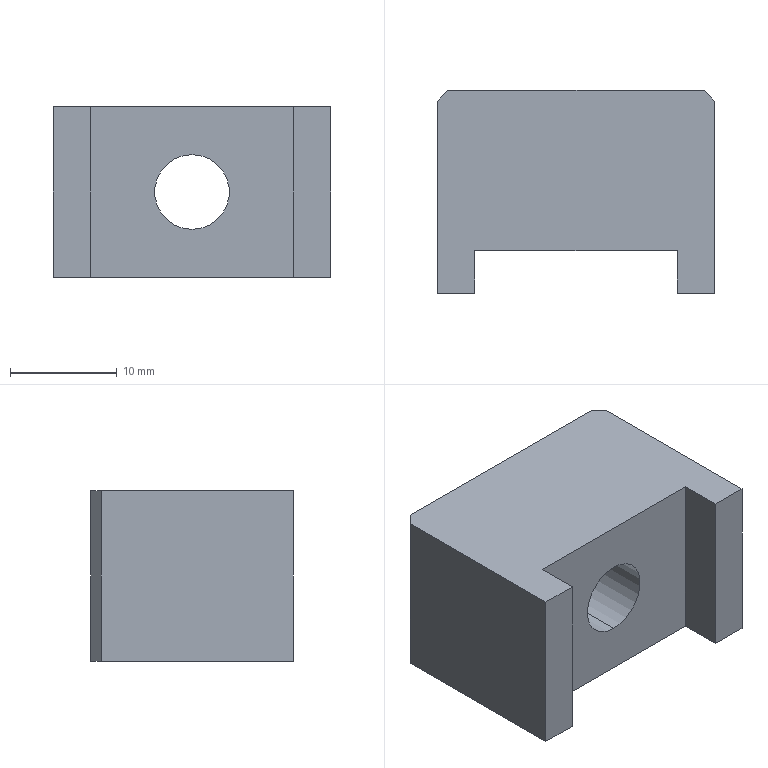Part | SolidWorks | features ICE 2, Chamfer 1, Extrusion 1 | 1 solid | 17 faces | box 26 x 19 x 16 mm | volume 5699 mm3 | plane 13 | cylinder 4 | commonest cylinder face diameters 7 x2 11 x2
STEP:
#1=CARTESIAN_POINT('',(13.,4.,4.5));
#2=VERTEX_POINT('',#1);
#3=CARTESIAN_POINT('',(13.,4.,11.5));
#4=VERTEX_POINT('',#3);
#5=CARTESIAN_POINT('',(13.,4.,8.));
#6=DIRECTION('',(0.,1.,0.));
#7=DIRECTION('',(0.,0.,1.));
#8=AXIS2_PLACEMENT_3D('',#5,#6,#7);
#9=CIRCLE('',#8,3.5);
#10=EDGE_CURVE('',#2,#4,#9,.T.);
#11=ORIENTED_EDGE('',*,*,#10,.F.);
#12=CARTESIAN_POINT('',(13.,12.,4.5));
#13=VERTEX_POINT('',#12);
#14=CARTESIAN_POINT('',(13.,4.,4.5));
#15=DIRECTION('',(0.,1.,0.));
#16=VECTOR('',#15,1000.);
#17=LINE('',#14,#16);
#18=EDGE_CURVE('',#2,#13,#17,.T.);
#19=ORIENTED_EDGE('',*,*,#18,.T.);
#20=CARTESIAN_POINT('',(13.,12.,11.5));
#21=VERTEX_POINT('',#20);
#22=CARTESIAN_POINT('',(13.,12.,8.));
#23=DIRECTION('',(0.,1.,0.));
#24=DIRECTION('',(0.,0.,1.));
#25=AXIS2_PLACEMENT_3D('',#22,#23,#24);
#26=CIRCLE('',#25,3.5);
#27=EDGE_CURVE('',#13,#21,#26,.T.);
#28=ORIENTED_EDGE('',*,*,#27,.T.);
#29=CARTESIAN_POINT('',(13.,4.,11.5));
#30=DIRECTION('',(0.,1.,0.));
#31=VECTOR('',#30,1000.);
#32=LINE('',#29,#31);
#33=EDGE_CURVE('',#4,#21,#32,.T.);
#34=ORIENTED_EDGE('',*,*,#33,.F.);
#35=EDGE_LOOP('',(#11,#19,#28,#34));
#36=FACE_OUTER_BOUND('',#35,.T.);
#37=CARTESIAN_POINT('',(13.,4.,8.));
#38=DIRECTION('',(0.,1.,0.));
#39=DIRECTION('',(0.,0.,1.));
#40=AXIS2_PLACEMENT_3D('',#37,#38,#39);
#41=CYLINDRICAL_SURFACE('',#40,3.5);
#42=ADVANCED_FACE('',(#36),#41,.F.);
#43=CARTESIAN_POINT('',(13.,12.,2.5));
#44=VERTEX_POINT('',#43);
#45=CARTESIAN_POINT('',(13.,12.,13.5));
#46=VERTEX_POINT('',#45);
#47=CARTESIAN_POINT('',(13.,12.,8.));
#48=DIRECTION('',(0.,1.,0.));
#49=DIRECTION('',(0.,0.,1.));
#50=AXIS2_PLACEMENT_3D('',#47,#48,#49);
#51=CIRCLE('',#50,5.5);
#52=EDGE_CURVE('',#44,#46,#51,.T.);
#53=ORIENTED_EDGE('',*,*,#52,.F.);
#54=CARTESIAN_POINT('',(13.,19.,2.5));
#55=VERTEX_POINT('',#54);
#56=CARTESIAN_POINT('',(13.,12.,2.5));
#57=DIRECTION('',(0.,1.,0.));
#58=VECTOR('',#57,1000.);
#59=LINE('',#56,#58);
#60=EDGE_CURVE('',#44,#55,#59,.T.);
#61=ORIENTED_EDGE('',*,*,#60,.T.);
#62=CARTESIAN_POINT('',(13.,19.,13.5));
#63=VERTEX_POINT('',#62);
#64=CARTESIAN_POINT('',(13.,19.,8.));
#65=DIRECTION('',(0.,1.,0.));
#66=DIRECTION('',(0.,0.,1.));
#67=AXIS2_PLACEMENT_3D('',#64,#65,#66);
#68=CIRCLE('',#67,5.5);
#69=EDGE_CURVE('',#55,#63,#68,.T.);
#70=ORIENTED_EDGE('',*,*,#69,.T.);
#71=CARTESIAN_POINT('',(13.,12.,13.5));
#72=DIRECTION('',(0.,1.,0.));
#73=VECTOR('',#72,1000.);
#74=LINE('',#71,#73);
#75=EDGE_CURVE('',#46,#63,#74,.T.);
#76=ORIENTED_EDGE('',*,*,#75,.F.);
#77=EDGE_LOOP('',(#53,#61,#70,#76));
#78=FACE_OUTER_BOUND('',#77,.T.);
#79=CARTESIAN_POINT('',(13.,12.,8.));
#80=DIRECTION('',(0.,1.,0.));
#81=DIRECTION('',(0.,0.,1.));
#82=AXIS2_PLACEMENT_3D('',#79,#80,#81);
#83=CYLINDRICAL_SURFACE('',#82,5.5);
#84=ADVANCED_FACE('',(#78),#83,.F.);
#85=CARTESIAN_POINT('',(0.,0.,0.));
#86=VERTEX_POINT('',#85);
#87=CARTESIAN_POINT('',(3.5,0.,0.));
#88=VERTEX_POINT('',#87);
#89=CARTESIAN_POINT('',(3.5,0.,0.));
#90=DIRECTION('',(1.,0.,0.));
#91=VECTOR('',#90,1000.);
#92=LINE('',#89,#91);
#93=EDGE_CURVE('',#86,#88,#92,.T.);
#94=ORIENTED_EDGE('',*,*,#93,.T.);
#95=CARTESIAN_POINT('',(3.5,0.,16.));
#96=VERTEX_POINT('',#95);
#97=CARTESIAN_POINT('',(3.5,0.,16.));
#98=DIRECTION('',(0.,0.,-1.));
#99=VECTOR('',#98,1000.);
#100=LINE('',#97,#99);
#101=EDGE_CURVE('',#96,#88,#100,.T.);
#102=ORIENTED_EDGE('',*,*,#101,.F.);
#103=CARTESIAN_POINT('',(0.,0.,16.));
#104=VERTEX_POINT('',#103);
#105=CARTESIAN_POINT('',(3.5,0.,16.));
#106=DIRECTION('',(1.,0.,0.));
#107=VECTOR('',#106,1000.);
#108=LINE('',#105,#107);
#109=EDGE_CURVE('',#104,#96,#108,.T.);
#110=ORIENTED_EDGE('',*,*,#109,.F.);
#111=CARTESIAN_POINT('',(0.,0.,16.));
#112=DIRECTION('',(0.,0.,-1.));
#113=VECTOR('',#112,1000.);
#114=LINE('',#111,#113);
#115=EDGE_CURVE('',#104,#86,#114,.T.);
#116=ORIENTED_EDGE('',*,*,#115,.T.);
#117=EDGE_LOOP('',(#94,#102,#110,#116));
#118=FACE_OUTER_BOUND('',#117,.T.);
#119=CARTESIAN_POINT('',(3.5,0.,16.));
#120=DIRECTION('',(0.,1.,0.));
#121=DIRECTION('',(-1.,0.,0.));
#122=AXIS2_PLACEMENT_3D('',#119,#120,#121);
#123=PLANE('',#122);
#124=ADVANCED_FACE('',(#118),#123,.F.);
#125=CARTESIAN_POINT('',(3.5,4.,0.));
#126=VERTEX_POINT('',#125);
#127=CARTESIAN_POINT('',(3.5,4.,0.));
#128=DIRECTION('',(0.,1.,0.));
#129=VECTOR('',#128,1000.);
#130=LINE('',#127,#129);
#131=EDGE_CURVE('',#88,#126,#130,.T.);
#132=ORIENTED_EDGE('',*,*,#131,.T.);
#133=CARTESIAN_POINT('',(3.5,4.,16.));
#134=VERTEX_POINT('',#133);
#135=CARTESIAN_POINT('',(3.5,4.,16.));
#136=DIRECTION('',(0.,0.,-1.));
#137=VECTOR('',#136,1000.);
#138=LINE('',#135,#137);
#139=EDGE_CURVE('',#134,#126,#138,.T.);
#140=ORIENTED_EDGE('',*,*,#139,.F.);
#141=CARTESIAN_POINT('',(3.5,4.,16.));
#142=DIRECTION('',(0.,1.,0.));
#143=VECTOR('',#142,1000.);
#144=LINE('',#141,#143);
#145=EDGE_CURVE('',#96,#134,#144,.T.);
#146=ORIENTED_EDGE('',*,*,#145,.F.);
#147=ORIENTED_EDGE('',*,*,#101,.T.);
#148=EDGE_LOOP('',(#132,#140,#146,#147));
#149=FACE_OUTER_BOUND('',#148,.T.);
#150=CARTESIAN_POINT('',(3.5,4.,16.));
#151=DIRECTION('',(-1.,0.,0.));
#152=DIRECTION('',(0.,-1.,0.));
#153=AXIS2_PLACEMENT_3D('',#150,#151,#152);
#154=PLANE('',#153);
#155=ADVANCED_FACE('',(#149),#154,.F.);
#156=CARTESIAN_POINT('',(13.,4.,8.));
#157=DIRECTION('',(0.,1.,0.));
#158=DIRECTION('',(0.,0.,1.));
#159=AXIS2_PLACEMENT_3D('',#156,#157,#158);
#160=CIRCLE('',#159,3.5);
#161=EDGE_CURVE('',#4,#2,#160,.T.);
#162=ORIENTED_EDGE('',*,*,#161,.T.);
#163=ORIENTED_EDGE('',*,*,#10,.T.);
#164=EDGE_LOOP('',(#162,#163));
#165=FACE_BOUND('',#164,.T.);
#166=CARTESIAN_POINT('',(22.5,4.,0.));
#167=VERTEX_POINT('',#166);
#168=CARTESIAN_POINT('',(22.5,4.,0.));
#169=DIRECTION('',(1.,0.,0.));
#170=VECTOR('',#169,1000.);
#171=LINE('',#168,#170);
#172=EDGE_CURVE('',#126,#167,#171,.T.);
#173=ORIENTED_EDGE('',*,*,#172,.T.);
#174=CARTESIAN_POINT('',(22.5,4.,16.));
#175=VERTEX_POINT('',#174);
#176=CARTESIAN_POINT('',(22.5,4.,16.));
#177=DIRECTION('',(0.,0.,-1.));
#178=VECTOR('',#177,1000.);
#179=LINE('',#176,#178);
#180=EDGE_CURVE('',#175,#167,#179,.T.);
#181=ORIENTED_EDGE('',*,*,#180,.F.);
#182=CARTESIAN_POINT('',(22.5,4.,16.));
#183=DIRECTION('',(1.,0.,0.));
#184=VECTOR('',#183,1000.);
#185=LINE('',#182,#184);
#186=EDGE_CURVE('',#134,#175,#185,.T.);
#187=ORIENTED_EDGE('',*,*,#186,.F.);
#188=ORIENTED_EDGE('',*,*,#139,.T.);
#189=EDGE_LOOP('',(#173,#181,#187,#188));
#190=FACE_OUTER_BOUND('',#189,.T.);
#191=CARTESIAN_POINT('',(22.5,4.,16.));
#192=DIRECTION('',(0.,1.,0.));
#193=DIRECTION('',(-1.,0.,0.));
#194=AXIS2_PLACEMENT_3D('',#191,#192,#193);
#195=PLANE('',#194);
#196=ADVANCED_FACE('',(#165,#190),#195,.F.);
#197=CARTESIAN_POINT('',(22.5,0.,0.));
#198=VERTEX_POINT('',#197);
#199=CARTESIAN_POINT('',(22.5,0.,0.));
#200=DIRECTION('',(0.,-1.,0.));
#201=VECTOR('',#200,1000.);
#202=LINE('',#199,#201);
#203=EDGE_CURVE('',#167,#198,#202,.T.);
#204=ORIENTED_EDGE('',*,*,#203,.T.);
#205=CARTESIAN_POINT('',(22.5,0.,16.));
#206=VERTEX_POINT('',#205);
#207=CARTESIAN_POINT('',(22.5,0.,16.));
#208=DIRECTION('',(0.,0.,-1.));
#209=VECTOR('',#208,1000.);
#210=LINE('',#207,#209);
#211=EDGE_CURVE('',#206,#198,#210,.T.);
#212=ORIENTED_EDGE('',*,*,#211,.F.);
#213=CARTESIAN_POINT('',(22.5,0.,16.));
#214=DIRECTION('',(0.,-1.,0.));
#215=VECTOR('',#214,1000.);
#216=LINE('',#213,#215);
#217=EDGE_CURVE('',#175,#206,#216,.T.);
#218=ORIENTED_EDGE('',*,*,#217,.F.);
#219=ORIENTED_EDGE('',*,*,#180,.T.);
#220=EDGE_LOOP('',(#204,#212,#218,#219));
#221=FACE_OUTER_BOUND('',#220,.T.);
#222=CARTESIAN_POINT('',(22.5,0.,16.));
#223=DIRECTION('',(1.,0.,0.));
#224=DIRECTION('',(0.,0.,-1.));
#225=AXIS2_PLACEMENT_3D('',#222,#223,#224);
#226=PLANE('',#225);
#227=ADVANCED_FACE('',(#221),#226,.F.);
#228=CARTESIAN_POINT('',(26.,0.,0.));
#229=VERTEX_POINT('',#228);
#230=CARTESIAN_POINT('',(26.,0.,0.));
#231=DIRECTION('',(1.,0.,0.));
#232=VECTOR('',#231,1000.);
#233=LINE('',#230,#232);
#234=EDGE_CURVE('',#198,#229,#233,.T.);
#235=ORIENTED_EDGE('',*,*,#234,.T.);
#236=CARTESIAN_POINT('',(26.,0.,16.));
#237=VERTEX_POINT('',#236);
#238=CARTESIAN_POINT('',(26.,0.,16.));
#239=DIRECTION('',(0.,0.,-1.));
#240=VECTOR('',#239,1000.);
#241=LINE('',#238,#240);
#242=EDGE_CURVE('',#237,#229,#241,.T.);
#243=ORIENTED_EDGE('',*,*,#242,.F.);
#244=CARTESIAN_POINT('',(26.,0.,16.));
#245=DIRECTION('',(1.,0.,0.));
#246=VECTOR('',#245,1000.);
#247=LINE('',#244,#246);
#248=EDGE_CURVE('',#206,#237,#247,.T.);
#249=ORIENTED_EDGE('',*,*,#248,.F.);
#250=ORIENTED_EDGE('',*,*,#211,.T.);
#251=EDGE_LOOP('',(#235,#243,#249,#250));
#252=FACE_OUTER_BOUND('',#251,.T.);
#253=CARTESIAN_POINT('',(26.,0.,16.));
#254=DIRECTION('',(0.,1.,0.));
#255=DIRECTION('',(-1.,0.,0.));
#256=AXIS2_PLACEMENT_3D('',#253,#254,#255);
#257=PLANE('',#256);
#258=ADVANCED_FACE('',(#252),#257,.F.);
#259=CARTESIAN_POINT('',(26.,18.,0.));
#260=VERTEX_POINT('',#259);
#261=CARTESIAN_POINT('',(26.,19.,0.));
#262=DIRECTION('',(0.,1.,0.));
#263=VECTOR('',#262,1000.);
#264=LINE('',#261,#263);
#265=EDGE_CURVE('',#229,#260,#264,.T.);
#266=ORIENTED_EDGE('',*,*,#265,.T.);
#267=CARTESIAN_POINT('',(26.,18.,16.));
#268=VERTEX_POINT('',#267);
#269=CARTESIAN_POINT('',(26.,18.,16.));
#270=DIRECTION('',(0.,0.,1.));
#271=VECTOR('',#270,1000.);
#272=LINE('',#269,#271);
#273=EDGE_CURVE('',#260,#268,#272,.T.);
#274=ORIENTED_EDGE('',*,*,#273,.T.);
#275=CARTESIAN_POINT('',(26.,19.,16.));
#276=DIRECTION('',(0.,1.,0.));
#277=VECTOR('',#276,1000.);
#278=LINE('',#275,#277);
#279=EDGE_CURVE('',#237,#268,#278,.T.);
#280=ORIENTED_EDGE('',*,*,#279,.F.);
#281=ORIENTED_EDGE('',*,*,#242,.T.);
#282=EDGE_LOOP('',(#266,#274,#280,#281));
#283=FACE_OUTER_BOUND('',#282,.T.);
#284=CARTESIAN_POINT('',(26.,19.,16.));
#285=DIRECTION('',(-1.,0.,0.));
#286=DIRECTION('',(0.,0.,1.));
#287=AXIS2_PLACEMENT_3D('',#284,#285,#286);
#288=PLANE('',#287);
#289=ADVANCED_FACE('',(#283),#288,.F.);
#290=CARTESIAN_POINT('',(13.,19.,8.));
#291=DIRECTION('',(0.,1.,0.));
#292=DIRECTION('',(0.,0.,1.));
#293=AXIS2_PLACEMENT_3D('',#290,#291,#292);
#294=CIRCLE('',#293,5.5);
#295=EDGE_CURVE('',#63,#55,#294,.T.);
#296=ORIENTED_EDGE('',*,*,#295,.F.);
#297=ORIENTED_EDGE('',*,*,#69,.F.);
#298=EDGE_LOOP('',(#296,#297));
#299=FACE_BOUND('',#298,.T.);
#300=CARTESIAN_POINT('',(25.,19.,16.));
#301=VERTEX_POINT('',#300);
#302=CARTESIAN_POINT('',(1.,19.,16.));
#303=VERTEX_POINT('',#302);
#304=CARTESIAN_POINT('',(0.,19.,16.));
#305=DIRECTION('',(-1.,0.,0.));
#306=VECTOR('',#305,1000.);
#307=LINE('',#304,#306);
#308=EDGE_CURVE('',#301,#303,#307,.T.);
#309=ORIENTED_EDGE('',*,*,#308,.F.);
#310=CARTESIAN_POINT('',(25.,19.,0.));
#311=VERTEX_POINT('',#310);
#312=CARTESIAN_POINT('',(25.,19.,16.));
#313=DIRECTION('',(0.,0.,-1.));
#314=VECTOR('',#313,1000.);
#315=LINE('',#312,#314);
#316=EDGE_CURVE('',#301,#311,#315,.T.);
#317=ORIENTED_EDGE('',*,*,#316,.T.);
#318=CARTESIAN_POINT('',(1.,19.,0.));
#319=VERTEX_POINT('',#318);
#320=CARTESIAN_POINT('',(0.,19.,0.));
#321=DIRECTION('',(-1.,0.,0.));
#322=VECTOR('',#321,1000.);
#323=LINE('',#320,#322);
#324=EDGE_CURVE('',#311,#319,#323,.T.);
#325=ORIENTED_EDGE('',*,*,#324,.T.);
#326=CARTESIAN_POINT('',(1.,19.,16.));
#327=DIRECTION('',(0.,0.,1.));
#328=VECTOR('',#327,1000.);
#329=LINE('',#326,#328);
#330=EDGE_CURVE('',#319,#303,#329,.T.);
#331=ORIENTED_EDGE('',*,*,#330,.T.);
#332=EDGE_LOOP('',(#309,#317,#325,#331));
#333=FACE_OUTER_BOUND('',#332,.T.);
#334=CARTESIAN_POINT('',(0.,19.,16.));
#335=DIRECTION('',(0.,-1.,0.));
#336=DIRECTION('',(0.,0.,-1.));
#337=AXIS2_PLACEMENT_3D('',#334,#335,#336);
#338=PLANE('',#337);
#339=ADVANCED_FACE('',(#299,#333),#338,.F.);
#340=CARTESIAN_POINT('',(0.,18.,16.));
#341=VERTEX_POINT('',#340);
#342=CARTESIAN_POINT('',(0.,0.,16.));
#343=DIRECTION('',(0.,-1.,0.));
#344=VECTOR('',#343,1000.);
#345=LINE('',#342,#344);
#346=EDGE_CURVE('',#341,#104,#345,.T.);
#347=ORIENTED_EDGE('',*,*,#346,.F.);
#348=CARTESIAN_POINT('',(0.,18.,0.));
#349=VERTEX_POINT('',#348);
#350=CARTESIAN_POINT('',(0.,18.,16.));
#351=DIRECTION('',(0.,0.,-1.));
#352=VECTOR('',#351,1000.);
#353=LINE('',#350,#352);
#354=EDGE_CURVE('',#341,#349,#353,.T.);
#355=ORIENTED_EDGE('',*,*,#354,.T.);
#356=CARTESIAN_POINT('',(0.,0.,0.));
#357=DIRECTION('',(0.,-1.,0.));
#358=VECTOR('',#357,1000.);
#359=LINE('',#356,#358);
#360=EDGE_CURVE('',#349,#86,#359,.T.);
#361=ORIENTED_EDGE('',*,*,#360,.T.);
#362=ORIENTED_EDGE('',*,*,#115,.F.);
#363=EDGE_LOOP('',(#347,#355,#361,#362));
#364=FACE_OUTER_BOUND('',#363,.T.);
#365=CARTESIAN_POINT('',(0.,0.,16.));
#366=DIRECTION('',(1.,0.,0.));
#367=DIRECTION('',(0.,0.,-1.));
#368=AXIS2_PLACEMENT_3D('',#365,#366,#367);
#369=PLANE('',#368);
#370=ADVANCED_FACE('',(#364),#369,.F.);
#371=ORIENTED_EDGE('',*,*,#279,.T.);
#372=CARTESIAN_POINT('',(25.,19.,16.));
#373=DIRECTION('',(-0.7071,0.7071,0.));
#374=VECTOR('',#373,1000.);
#375=LINE('',#372,#374);
#376=EDGE_CURVE('',#268,#301,#375,.T.);
#377=ORIENTED_EDGE('',*,*,#376,.T.);
#378=ORIENTED_EDGE('',*,*,#308,.T.);
#379=CARTESIAN_POINT('',(0.,18.,16.));
#380=DIRECTION('',(-0.7071,-0.7071,0.));
#381=VECTOR('',#380,1000.);
#382=LINE('',#379,#381);
#383=EDGE_CURVE('',#303,#341,#382,.T.);
#384=ORIENTED_EDGE('',*,*,#383,.T.);
#385=ORIENTED_EDGE('',*,*,#346,.T.);
#386=ORIENTED_EDGE('',*,*,#109,.T.);
#387=ORIENTED_EDGE('',*,*,#145,.T.);
#388=ORIENTED_EDGE('',*,*,#186,.T.);
#389=ORIENTED_EDGE('',*,*,#217,.T.);
#390=ORIENTED_EDGE('',*,*,#248,.T.);
#391=EDGE_LOOP('',(#371,#377,#378,#384,#385,#386,#387,#388,#389,#390));
#392=FACE_OUTER_BOUND('',#391,.T.);
#393=CARTESIAN_POINT('',(0.,0.,16.));
#394=DIRECTION('',(0.,0.,-1.));
#395=DIRECTION('',(-1.,0.,0.));
#396=AXIS2_PLACEMENT_3D('',#393,#394,#395);
#397=PLANE('',#396);
#398=ADVANCED_FACE('',(#392),#397,.F.);
#399=ORIENTED_EDGE('',*,*,#324,.F.);
#400=CARTESIAN_POINT('',(22.,22.,0.));
#401=DIRECTION('',(0.7071,-0.7071,0.));
#402=VECTOR('',#401,1000.);
#403=LINE('',#400,#402);
#404=EDGE_CURVE('',#311,#260,#403,.T.);
#405=ORIENTED_EDGE('',*,*,#404,.T.);
#406=ORIENTED_EDGE('',*,*,#265,.F.);
#407=ORIENTED_EDGE('',*,*,#234,.F.);
#408=ORIENTED_EDGE('',*,*,#203,.F.);
#409=ORIENTED_EDGE('',*,*,#172,.F.);
#410=ORIENTED_EDGE('',*,*,#131,.F.);
#411=ORIENTED_EDGE('',*,*,#93,.F.);
#412=ORIENTED_EDGE('',*,*,#360,.F.);
#413=CARTESIAN_POINT('',(-9.,9.,0.));
#414=DIRECTION('',(0.7071,0.7071,0.));
#415=VECTOR('',#414,1000.);
#416=LINE('',#413,#415);
#417=EDGE_CURVE('',#349,#319,#416,.T.);
#418=ORIENTED_EDGE('',*,*,#417,.T.);
#419=EDGE_LOOP('',(#399,#405,#406,#407,#408,#409,#410,#411,#412,#418));
#420=FACE_OUTER_BOUND('',#419,.T.);
#421=CARTESIAN_POINT('',(0.,0.,0.));
#422=DIRECTION('',(0.,0.,-1.));
#423=DIRECTION('',(-1.,0.,0.));
#424=AXIS2_PLACEMENT_3D('',#421,#422,#423);
#425=PLANE('',#424);
#426=ADVANCED_FACE('',(#420),#425,.T.);
#427=ORIENTED_EDGE('',*,*,#60,.F.);
#428=CARTESIAN_POINT('',(13.,12.,8.));
#429=DIRECTION('',(0.,1.,0.));
#430=DIRECTION('',(0.,0.,1.));
#431=AXIS2_PLACEMENT_3D('',#428,#429,#430);
#432=CIRCLE('',#431,5.5);
#433=EDGE_CURVE('',#46,#44,#432,.T.);
#434=ORIENTED_EDGE('',*,*,#433,.F.);
#435=ORIENTED_EDGE('',*,*,#75,.T.);
#436=ORIENTED_EDGE('',*,*,#295,.T.);
#437=EDGE_LOOP('',(#427,#434,#435,#436));
#438=FACE_OUTER_BOUND('',#437,.T.);
#439=CARTESIAN_POINT('',(13.,12.,8.));
#440=DIRECTION('',(0.,1.,0.));
#441=DIRECTION('',(0.,0.,1.));
#442=AXIS2_PLACEMENT_3D('',#439,#440,#441);
#443=CYLINDRICAL_SURFACE('',#442,5.5);
#444=ADVANCED_FACE('',(#438),#443,.F.);
#445=CARTESIAN_POINT('',(13.,12.,8.));
#446=DIRECTION('',(0.,1.,0.));
#447=DIRECTION('',(0.,0.,1.));
#448=AXIS2_PLACEMENT_3D('',#445,#446,#447);
#449=CIRCLE('',#448,3.5);
#450=EDGE_CURVE('',#21,#13,#449,.T.);
#451=ORIENTED_EDGE('',*,*,#450,.F.);
#452=ORIENTED_EDGE('',*,*,#27,.F.);
#453=EDGE_LOOP('',(#451,#452));
#454=FACE_BOUND('',#453,.T.);
#455=ORIENTED_EDGE('',*,*,#433,.T.);
#456=ORIENTED_EDGE('',*,*,#52,.T.);
#457=EDGE_LOOP('',(#455,#456));
#458=FACE_OUTER_BOUND('',#457,.T.);
#459=CARTESIAN_POINT('',(13.,12.,8.));
#460=DIRECTION('',(0.,1.,0.));
#461=DIRECTION('',(0.,0.,1.));
#462=AXIS2_PLACEMENT_3D('',#459,#460,#461);
#463=PLANE('',#462);
#464=ADVANCED_FACE('',(#454,#458),#463,.T.);
#465=ORIENTED_EDGE('',*,*,#18,.F.);
#466=ORIENTED_EDGE('',*,*,#161,.F.);
#467=ORIENTED_EDGE('',*,*,#33,.T.);
#468=ORIENTED_EDGE('',*,*,#450,.T.);
#469=EDGE_LOOP('',(#465,#466,#467,#468));
#470=FACE_OUTER_BOUND('',#469,.T.);
#471=CARTESIAN_POINT('',(13.,4.,8.));
#472=DIRECTION('',(0.,1.,0.));
#473=DIRECTION('',(0.,0.,1.));
#474=AXIS2_PLACEMENT_3D('',#471,#472,#473);
#475=CYLINDRICAL_SURFACE('',#474,3.5);
#476=ADVANCED_FACE('',(#470),#475,.F.);
#477=ORIENTED_EDGE('',*,*,#376,.F.);
#478=ORIENTED_EDGE('',*,*,#273,.F.);
#479=ORIENTED_EDGE('',*,*,#404,.F.);
#480=ORIENTED_EDGE('',*,*,#316,.F.);
#481=EDGE_LOOP('',(#477,#478,#479,#480));
#482=FACE_OUTER_BOUND('',#481,.T.);
#483=CARTESIAN_POINT('',(25.,19.,16.));
#484=DIRECTION('',(-0.7071,-0.7071,0.));
#485=DIRECTION('',(0.,0.,-1.));
#486=AXIS2_PLACEMENT_3D('',#483,#484,#485);
#487=PLANE('',#486);
#488=ADVANCED_FACE('',(#482),#487,.F.);
#489=ORIENTED_EDGE('',*,*,#383,.F.);
#490=ORIENTED_EDGE('',*,*,#330,.F.);
#491=ORIENTED_EDGE('',*,*,#417,.F.);
#492=ORIENTED_EDGE('',*,*,#354,.F.);
#493=EDGE_LOOP('',(#489,#490,#491,#492));
#494=FACE_OUTER_BOUND('',#493,.T.);
#495=CARTESIAN_POINT('',(0.,18.,16.));
#496=DIRECTION('',(0.7071,-0.7071,0.));
#497=DIRECTION('',(0.,0.,-1.));
#498=AXIS2_PLACEMENT_3D('',#495,#496,#497);
#499=PLANE('',#498);
#500=ADVANCED_FACE('',(#494),#499,.F.);
#501=CLOSED_SHELL('',(#42,#84,#124,#155,#196,#227,#258,#289,#339,#370,#398,#426,#444,#464,#476,#488,#500));
#502=MANIFOLD_SOLID_BREP('',#501);
#503=CARTESIAN_POINT('',(0.,0.,0.));
#504=DIRECTION('',(0.,0.,1.));
#505=DIRECTION('',(1.,0.,0.));
#506=AXIS2_PLACEMENT_3D('',#503,#504,#505);
#507=(LENGTH_UNIT()NAMED_UNIT(*)SI_UNIT(.MILLI.,.METRE.));
#508=UNCERTAINTY_MEASURE_WITH_UNIT(LENGTH_MEASURE(0.00001),#507,'','');
#509=(NAMED_UNIT(*)PLANE_ANGLE_UNIT()SI_UNIT($,.RADIAN.));
#510=(NAMED_UNIT(*)SI_UNIT($,.STERADIAN.)SOLID_ANGLE_UNIT());
#511=(GEOMETRIC_REPRESENTATION_CONTEXT(3)GLOBAL_UNCERTAINTY_ASSIGNED_CONTEXT((#508))GLOBAL_UNIT_ASSIGNED_CONTEXT((#507,#509,#510))REPRESENTATION_CONTEXT('',''));
#512=ADVANCED_BREP_SHAPE_REPRESENTATION('',(#502,#506),#511);